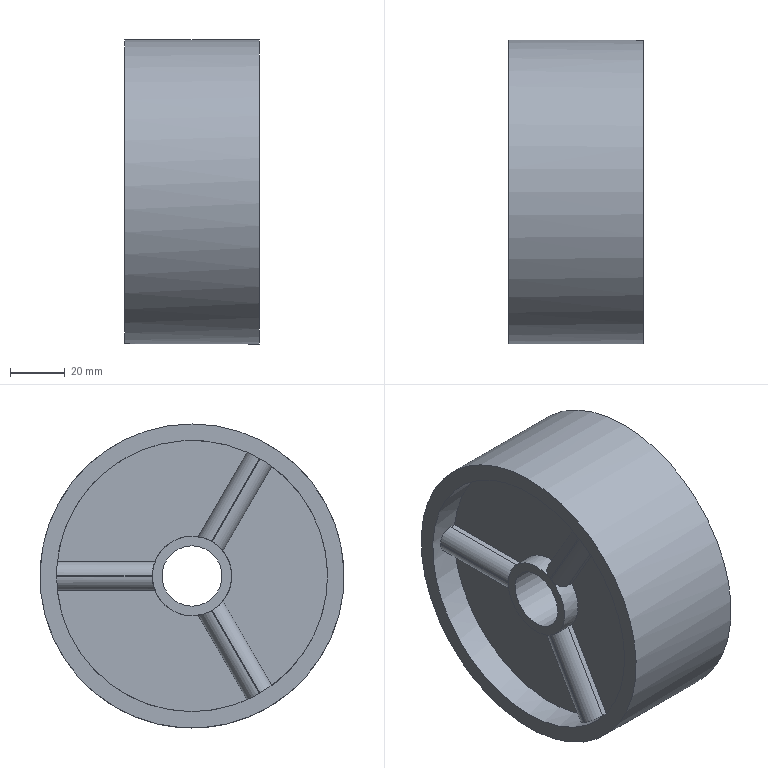Part | NX | features EXTRUDE 3, BLEND 1, DATUM_CSYS 1, EXTRACT_DATUM_PLANE 1, SKETCH 1, UNITE 1 | 1 solid | 44 faces | box 49 x 111 x 111 mm | volume 318902 mm3 | plane 22 | cylinder 22 | commonest cylinder face diameters 10 x12 29.03 x6 99 x2 22 x1 111 x1
STEP:
#1=CARTESIAN_POINT('',(-13.797,-29.113,40.033));
#2=VERTEX_POINT('',#1);
#3=CARTESIAN_POINT('',(-15.797,-29.113,40.033));
#4=VERTEX_POINT('',#3);
#5=CARTESIAN_POINT('',(21.203,-29.113,40.033));
#6=DIRECTION('',(-1.,0.,0.));
#7=VECTOR('',#6,1000.);
#8=LINE('',#5,#7);
#9=EDGE_CURVE('',#2,#4,#8,.T.);
#10=ORIENTED_EDGE('',*,*,#9,.T.);
#11=CARTESIAN_POINT('',(-15.797,-11.277,9.139));
#12=VERTEX_POINT('',#11);
#13=CARTESIAN_POINT('',(-15.797,-11.277,9.139));
#14=DIRECTION('',(0.,-0.5,0.866));
#15=VECTOR('',#14,1000.);
#16=LINE('',#13,#15);
#17=EDGE_CURVE('',#4,#12,#16,.F.);
#18=ORIENTED_EDGE('',*,*,#17,.T.);
#19=CARTESIAN_POINT('',(-13.797,-11.277,9.139));
#20=VERTEX_POINT('',#19);
#21=CARTESIAN_POINT('',(21.203,-11.277,9.139));
#22=DIRECTION('',(-1.,0.,0.));
#23=VECTOR('',#22,1000.);
#24=LINE('',#21,#23);
#25=EDGE_CURVE('',#20,#12,#24,.T.);
#26=ORIENTED_EDGE('',*,*,#25,.F.);
#27=CARTESIAN_POINT('',(-13.797,-29.113,40.033));
#28=DIRECTION('',(0.,0.5,-0.866));
#29=VECTOR('',#28,1000.);
#30=LINE('',#27,#29);
#31=EDGE_CURVE('',#2,#20,#30,.T.);
#32=ORIENTED_EDGE('',*,*,#31,.F.);
#33=EDGE_LOOP('',(#10,#18,#26,#32));
#34=FACE_BOUND('',#33,.T.);
#35=CARTESIAN_POINT('',(21.203,-11.277,9.139));
#36=DIRECTION('',(0.,-0.866,-0.5));
#37=DIRECTION('',(0.,0.5,-0.866));
#38=AXIS2_PLACEMENT_3D('',#35,#36,#37);
#39=PLANE('',#38);
#40=ADVANCED_FACE('',(#34),#39,.T.);
#41=CARTESIAN_POINT('',(-13.797,-11.277,-9.139));
#42=VERTEX_POINT('',#41);
#43=CARTESIAN_POINT('',(-15.797,-11.277,-9.139));
#44=VERTEX_POINT('',#43);
#45=CARTESIAN_POINT('',(21.203,-11.277,-9.139));
#46=DIRECTION('',(-1.,0.,0.));
#47=VECTOR('',#46,1000.);
#48=LINE('',#45,#47);
#49=EDGE_CURVE('',#42,#44,#48,.T.);
#50=ORIENTED_EDGE('',*,*,#49,.T.);
#51=CARTESIAN_POINT('',(-15.797,-29.113,-40.033));
#52=VERTEX_POINT('',#51);
#53=CARTESIAN_POINT('',(-15.797,-29.113,-40.033));
#54=DIRECTION('',(0.,0.5,0.866));
#55=VECTOR('',#54,1000.);
#56=LINE('',#53,#55);
#57=EDGE_CURVE('',#44,#52,#56,.F.);
#58=ORIENTED_EDGE('',*,*,#57,.T.);
#59=CARTESIAN_POINT('',(-13.797,-29.113,-40.033));
#60=VERTEX_POINT('',#59);
#61=CARTESIAN_POINT('',(21.203,-29.113,-40.033));
#62=DIRECTION('',(-1.,0.,0.));
#63=VECTOR('',#62,1000.);
#64=LINE('',#61,#63);
#65=EDGE_CURVE('',#60,#52,#64,.T.);
#66=ORIENTED_EDGE('',*,*,#65,.F.);
#67=CARTESIAN_POINT('',(-13.797,-11.277,-9.139));
#68=DIRECTION('',(0.,-0.5,-0.866));
#69=VECTOR('',#68,1000.);
#70=LINE('',#67,#69);
#71=EDGE_CURVE('',#42,#60,#70,.T.);
#72=ORIENTED_EDGE('',*,*,#71,.F.);
#73=EDGE_LOOP('',(#50,#58,#66,#72));
#74=FACE_BOUND('',#73,.T.);
#75=CARTESIAN_POINT('',(21.203,-29.113,-40.033));
#76=DIRECTION('',(0.,-0.866,0.5));
#77=DIRECTION('',(0.,-0.5,-0.866));
#78=AXIS2_PLACEMENT_3D('',#75,#76,#77);
#79=PLANE('',#78);
#80=ADVANCED_FACE('',(#74),#79,.T.);
#81=CARTESIAN_POINT('',(-24.797,0.,-49.5));
#82=VERTEX_POINT('',#81);
#83=CARTESIAN_POINT('',(-24.797,0.,0.));
#84=DIRECTION('',(1.,0.,0.));
#85=DIRECTION('',(0.,0.,-1.));
#86=AXIS2_PLACEMENT_3D('',#83,#84,#85);
#87=CIRCLE('',#86,49.5);
#88=EDGE_CURVE('',#82,#82,#87,.T.);
#89=ORIENTED_EDGE('',*,*,#88,.F.);
#90=EDGE_LOOP('',(#89));
#91=FACE_BOUND('',#90,.T.);
#92=CARTESIAN_POINT('',(-13.797,0.,0.));
#93=DIRECTION('',(-1.,0.,0.));
#94=DIRECTION('',(0.,0.,1.));
#95=AXIS2_PLACEMENT_3D('',#92,#93,#94);
#96=CIRCLE('',#95,49.5);
#97=EDGE_CURVE('',#60,#2,#96,.T.);
#98=ORIENTED_EDGE('',*,*,#97,.F.);
#99=ORIENTED_EDGE('',*,*,#65,.T.);
#100=CARTESIAN_POINT('',(-20.797,-24.92,-42.77));
#101=VERTEX_POINT('',#100);
#102=CARTESIAN_POINT('',(-15.797,-29.113,-40.033));
#103=CARTESIAN_POINT('',(-17.119,-29.113,-40.033));
#104=CARTESIAN_POINT('',(-19.705,-28.237,-40.691));
#105=CARTESIAN_POINT('',(-20.797,-26.062,-42.105));
#106=CARTESIAN_POINT('',(-20.797,-24.92,-42.77));
#107=B_SPLINE_CURVE_WITH_KNOTS('',3,(#102,#103,#104,#105,#106),.UNSPECIFIED.,.F.,.F.,(4,1,4),(0.,0.003908,0.007816),.UNSPECIFIED.);
#108=EDGE_CURVE('',#52,#101,#107,.T.);
#109=ORIENTED_EDGE('',*,*,#108,.T.);
#110=CARTESIAN_POINT('',(-20.797,-24.58,-42.966));
#111=VERTEX_POINT('',#110);
#112=CARTESIAN_POINT('',(-20.797,0.,0.));
#113=DIRECTION('',(-1.,0.,0.));
#114=DIRECTION('',(0.,0.,1.));
#115=AXIS2_PLACEMENT_3D('',#112,#113,#114);
#116=CIRCLE('',#115,49.5);
#117=EDGE_CURVE('',#111,#101,#116,.T.);
#118=ORIENTED_EDGE('',*,*,#117,.F.);
#119=CARTESIAN_POINT('',(-15.797,-20.113,-45.229));
#120=VERTEX_POINT('',#119);
#121=CARTESIAN_POINT('',(-20.797,-24.58,-42.966));
#122=CARTESIAN_POINT('',(-20.797,-23.433,-43.622));
#123=CARTESIAN_POINT('',(-19.71,-21.125,-44.797));
#124=CARTESIAN_POINT('',(-17.119,-20.113,-45.229));
#125=CARTESIAN_POINT('',(-15.797,-20.113,-45.229));
#126=B_SPLINE_CURVE_WITH_KNOTS('',3,(#121,#122,#123,#124,#125),.UNSPECIFIED.,.F.,.F.,(4,1,4),(0.,0.003908,0.007816),.UNSPECIFIED.);
#127=EDGE_CURVE('',#111,#120,#126,.T.);
#128=ORIENTED_EDGE('',*,*,#127,.T.);
#129=CARTESIAN_POINT('',(-13.797,-20.113,-45.229));
#130=VERTEX_POINT('',#129);
#131=CARTESIAN_POINT('',(21.203,-20.113,-45.229));
#132=DIRECTION('',(-1.,0.,0.));
#133=VECTOR('',#132,1000.);
#134=LINE('',#131,#133);
#135=EDGE_CURVE('',#130,#120,#134,.T.);
#136=ORIENTED_EDGE('',*,*,#135,.F.);
#137=CARTESIAN_POINT('',(-13.797,49.227,-5.196));
#138=VERTEX_POINT('',#137);
#139=CARTESIAN_POINT('',(-13.797,0.,0.));
#140=DIRECTION('',(-1.,0.,0.));
#141=DIRECTION('',(0.,0.,1.));
#142=AXIS2_PLACEMENT_3D('',#139,#140,#141);
#143=CIRCLE('',#142,49.5);
#144=EDGE_CURVE('',#138,#130,#143,.T.);
#145=ORIENTED_EDGE('',*,*,#144,.F.);
#146=CARTESIAN_POINT('',(-15.797,49.227,-5.196));
#147=VERTEX_POINT('',#146);
#148=CARTESIAN_POINT('',(21.203,49.227,-5.196));
#149=DIRECTION('',(-1.,0.,0.));
#150=VECTOR('',#149,1000.);
#151=LINE('',#148,#150);
#152=EDGE_CURVE('',#138,#147,#151,.T.);
#153=ORIENTED_EDGE('',*,*,#152,.T.);
#154=CARTESIAN_POINT('',(-20.797,49.5,-0.1962));
#155=VERTEX_POINT('',#154);
#156=CARTESIAN_POINT('',(-15.797,49.227,-5.196));
#157=CARTESIAN_POINT('',(-17.119,49.227,-5.196));
#158=CARTESIAN_POINT('',(-19.705,49.358,-4.109));
#159=CARTESIAN_POINT('',(-20.797,49.494,-1.518));
#160=CARTESIAN_POINT('',(-20.797,49.5,-0.1962));
#161=B_SPLINE_CURVE_WITH_KNOTS('',3,(#156,#157,#158,#159,#160),.UNSPECIFIED.,.F.,.F.,(4,1,4),(0.,0.003908,0.007816),.UNSPECIFIED.);
#162=EDGE_CURVE('',#147,#155,#161,.T.);
#163=ORIENTED_EDGE('',*,*,#162,.T.);
#164=CARTESIAN_POINT('',(-20.797,49.5,0.1962));
#165=VERTEX_POINT('',#164);
#166=CARTESIAN_POINT('',(-20.797,0.,0.));
#167=DIRECTION('',(-1.,0.,0.));
#168=DIRECTION('',(0.,0.,-1.));
#169=AXIS2_PLACEMENT_3D('',#166,#167,#168);
#170=CIRCLE('',#169,49.5);
#171=EDGE_CURVE('',#165,#155,#170,.T.);
#172=ORIENTED_EDGE('',*,*,#171,.F.);
#173=CARTESIAN_POINT('',(-15.797,49.227,5.196));
#174=VERTEX_POINT('',#173);
#175=CARTESIAN_POINT('',(-20.797,49.5,0.1962));
#176=CARTESIAN_POINT('',(-20.797,49.494,1.518));
#177=CARTESIAN_POINT('',(-19.71,49.358,4.104));
#178=CARTESIAN_POINT('',(-17.119,49.227,5.196));
#179=CARTESIAN_POINT('',(-15.797,49.227,5.196));
#180=B_SPLINE_CURVE_WITH_KNOTS('',3,(#175,#176,#177,#178,#179),.UNSPECIFIED.,.F.,.F.,(4,1,4),(0.,0.003908,0.007816),.UNSPECIFIED.);
#181=EDGE_CURVE('',#165,#174,#180,.T.);
#182=ORIENTED_EDGE('',*,*,#181,.T.);
#183=CARTESIAN_POINT('',(-13.797,49.227,5.196));
#184=VERTEX_POINT('',#183);
#185=CARTESIAN_POINT('',(21.203,49.227,5.196));
#186=DIRECTION('',(-1.,0.,0.));
#187=VECTOR('',#186,1000.);
#188=LINE('',#185,#187);
#189=EDGE_CURVE('',#184,#174,#188,.T.);
#190=ORIENTED_EDGE('',*,*,#189,.F.);
#191=CARTESIAN_POINT('',(-13.797,-20.113,45.229));
#192=VERTEX_POINT('',#191);
#193=CARTESIAN_POINT('',(-13.797,0.,0.));
#194=DIRECTION('',(-1.,0.,0.));
#195=DIRECTION('',(0.,0.,-1.));
#196=AXIS2_PLACEMENT_3D('',#193,#194,#195);
#197=CIRCLE('',#196,49.5);
#198=EDGE_CURVE('',#192,#184,#197,.T.);
#199=ORIENTED_EDGE('',*,*,#198,.F.);
#200=CARTESIAN_POINT('',(-15.797,-20.113,45.229));
#201=VERTEX_POINT('',#200);
#202=CARTESIAN_POINT('',(21.203,-20.113,45.229));
#203=DIRECTION('',(-1.,0.,0.));
#204=VECTOR('',#203,1000.);
#205=LINE('',#202,#204);
#206=EDGE_CURVE('',#192,#201,#205,.T.);
#207=ORIENTED_EDGE('',*,*,#206,.T.);
#208=CARTESIAN_POINT('',(-20.797,-24.58,42.966));
#209=VERTEX_POINT('',#208);
#210=CARTESIAN_POINT('',(-15.797,-20.113,45.229));
#211=CARTESIAN_POINT('',(-17.119,-20.113,45.229));
#212=CARTESIAN_POINT('',(-19.705,-21.121,44.799));
#213=CARTESIAN_POINT('',(-20.797,-23.433,43.622));
#214=CARTESIAN_POINT('',(-20.797,-24.58,42.966));
#215=B_SPLINE_CURVE_WITH_KNOTS('',3,(#210,#211,#212,#213,#214),.UNSPECIFIED.,.F.,.F.,(4,1,4),(0.,0.003908,0.007816),.UNSPECIFIED.);
#216=EDGE_CURVE('',#201,#209,#215,.T.);
#217=ORIENTED_EDGE('',*,*,#216,.T.);
#218=CARTESIAN_POINT('',(-20.797,-24.92,42.77));
#219=VERTEX_POINT('',#218);
#220=CARTESIAN_POINT('',(-20.797,0.,0.));
#221=DIRECTION('',(-1.,0.,0.));
#222=DIRECTION('',(0.,0.,1.));
#223=AXIS2_PLACEMENT_3D('',#220,#221,#222);
#224=CIRCLE('',#223,49.5);
#225=EDGE_CURVE('',#219,#209,#224,.T.);
#226=ORIENTED_EDGE('',*,*,#225,.F.);
#227=CARTESIAN_POINT('',(-20.797,-24.92,42.77));
#228=CARTESIAN_POINT('',(-20.797,-26.062,42.105));
#229=CARTESIAN_POINT('',(-19.71,-28.233,40.693));
#230=CARTESIAN_POINT('',(-17.119,-29.113,40.033));
#231=CARTESIAN_POINT('',(-15.797,-29.113,40.033));
#232=B_SPLINE_CURVE_WITH_KNOTS('',3,(#227,#228,#229,#230,#231),.UNSPECIFIED.,.F.,.F.,(4,1,4),(0.,0.003908,0.007816),.UNSPECIFIED.);
#233=EDGE_CURVE('',#219,#4,#232,.T.);
#234=ORIENTED_EDGE('',*,*,#233,.T.);
#235=ORIENTED_EDGE('',*,*,#9,.F.);
#236=EDGE_LOOP('',(#98,#99,#109,#118,#128,#136,#145,#153,#163,#172,#182,#190,#199,#207,#217,#226,#234,#235));
#237=FACE_BOUND('',#236,.T.);
#238=CARTESIAN_POINT('',(24.203,0.,0.));
#239=DIRECTION('',(-1.,0.,0.));
#240=DIRECTION('',(0.,0.,1.));
#241=AXIS2_PLACEMENT_3D('',#238,#239,#240);
#242=CYLINDRICAL_SURFACE('',#241,49.5);
#243=ADVANCED_FACE('',(#91,#237),#242,.F.);
#244=CARTESIAN_POINT('',(-13.797,0.,0.));
#245=DIRECTION('',(1.,0.,0.));
#246=DIRECTION('',(0.,-0.7769,0.6296));
#247=AXIS2_PLACEMENT_3D('',#244,#245,#246);
#248=CIRCLE('',#247,14.515);
#249=EDGE_CURVE('',#20,#42,#248,.T.);
#250=ORIENTED_EDGE('',*,*,#249,.F.);
#251=ORIENTED_EDGE('',*,*,#25,.T.);
#252=CARTESIAN_POINT('',(-20.797,-7.427,12.471));
#253=VERTEX_POINT('',#252);
#254=CARTESIAN_POINT('',(-15.797,-11.277,9.139));
#255=CARTESIAN_POINT('',(-17.131,-11.277,9.139));
#256=CARTESIAN_POINT('',(-19.701,-10.567,10.1));
#257=CARTESIAN_POINT('',(-20.797,-8.572,11.789));
#258=CARTESIAN_POINT('',(-20.797,-7.427,12.471));
#259=B_SPLINE_CURVE_WITH_KNOTS('',3,(#254,#255,#256,#257,#258),.UNSPECIFIED.,.F.,.F.,(4,1,4),(0.,0.00394,0.00788),.UNSPECIFIED.);
#260=EDGE_CURVE('',#12,#253,#259,.T.);
#261=ORIENTED_EDGE('',*,*,#260,.T.);
#262=CARTESIAN_POINT('',(-20.797,-7.427,-12.471));
#263=VERTEX_POINT('',#262);
#264=CARTESIAN_POINT('',(-20.797,0.,0.));
#265=DIRECTION('',(-1.,0.,0.));
#266=DIRECTION('',(0.,-0.7769,0.6296));
#267=AXIS2_PLACEMENT_3D('',#264,#265,#266);
#268=CIRCLE('',#267,14.515);
#269=EDGE_CURVE('',#263,#253,#268,.T.);
#270=ORIENTED_EDGE('',*,*,#269,.F.);
#271=CARTESIAN_POINT('',(-20.797,-7.427,-12.471));
#272=CARTESIAN_POINT('',(-20.797,-8.572,-11.789));
#273=CARTESIAN_POINT('',(-19.703,-10.565,-10.101));
#274=CARTESIAN_POINT('',(-17.131,-11.277,-9.139));
#275=CARTESIAN_POINT('',(-15.797,-11.277,-9.139));
#276=B_SPLINE_CURVE_WITH_KNOTS('',3,(#271,#272,#273,#274,#275),.UNSPECIFIED.,.F.,.F.,(4,1,4),(0.,0.00394,0.007881),.UNSPECIFIED.);
#277=EDGE_CURVE('',#263,#44,#276,.T.);
#278=ORIENTED_EDGE('',*,*,#277,.T.);
#279=ORIENTED_EDGE('',*,*,#49,.F.);
#280=EDGE_LOOP('',(#250,#251,#261,#270,#278,#279));
#281=FACE_BOUND('',#280,.T.);
#282=CARTESIAN_POINT('',(21.203,0.,0.));
#283=DIRECTION('',(-1.,0.,0.));
#284=DIRECTION('',(0.,0.,1.));
#285=AXIS2_PLACEMENT_3D('',#282,#283,#284);
#286=CYLINDRICAL_SURFACE('',#285,14.515);
#287=ADVANCED_FACE('',(#281),#286,.T.);
#288=CARTESIAN_POINT('',(-24.797,0.,55.5));
#289=VERTEX_POINT('',#288);
#290=CARTESIAN_POINT('',(-24.797,0.,0.));
#291=DIRECTION('',(-1.,0.,0.));
#292=DIRECTION('',(0.,0.,1.));
#293=AXIS2_PLACEMENT_3D('',#290,#291,#292);
#294=CIRCLE('',#293,55.5);
#295=EDGE_CURVE('',#289,#289,#294,.T.);
#296=ORIENTED_EDGE('',*,*,#295,.F.);
#297=EDGE_LOOP('',(#296));
#298=FACE_BOUND('',#297,.T.);
#299=CARTESIAN_POINT('',(24.203,0.,-55.5));
#300=VERTEX_POINT('',#299);
#301=CARTESIAN_POINT('',(24.203,0.,0.));
#302=DIRECTION('',(-1.,0.,0.));
#303=DIRECTION('',(0.,0.,-1.));
#304=AXIS2_PLACEMENT_3D('',#301,#302,#303);
#305=CIRCLE('',#304,55.5);
#306=EDGE_CURVE('',#300,#300,#305,.T.);
#307=ORIENTED_EDGE('',*,*,#306,.T.);
#308=EDGE_LOOP('',(#307));
#309=FACE_BOUND('',#308,.T.);
#310=CARTESIAN_POINT('',(24.203,0.,0.));
#311=DIRECTION('',(-1.,0.,0.));
#312=DIRECTION('',(0.,0.,1.));
#313=AXIS2_PLACEMENT_3D('',#310,#311,#312);
#314=CYLINDRICAL_SURFACE('',#313,55.5);
#315=ADVANCED_FACE('',(#298,#309),#314,.T.);
#316=CARTESIAN_POINT('',(21.203,-24.58,-42.966));
#317=VERTEX_POINT('',#316);
#318=CARTESIAN_POINT('',(21.203,-24.92,-42.77));
#319=VERTEX_POINT('',#318);
#320=CARTESIAN_POINT('',(21.203,0.,0.));
#321=DIRECTION('',(-1.,0.,0.));
#322=DIRECTION('',(0.,0.,1.));
#323=AXIS2_PLACEMENT_3D('',#320,#321,#322);
#324=CIRCLE('',#323,49.5);
#325=EDGE_CURVE('',#317,#319,#324,.T.);
#326=ORIENTED_EDGE('',*,*,#325,.T.);
#327=CARTESIAN_POINT('',(16.203,-29.113,-40.033));
#328=VERTEX_POINT('',#327);
#329=CARTESIAN_POINT('',(21.203,-24.92,-42.77));
#330=CARTESIAN_POINT('',(21.203,-26.062,-42.105));
#331=CARTESIAN_POINT('',(20.116,-28.233,-40.693));
#332=CARTESIAN_POINT('',(17.524,-29.113,-40.033));
#333=CARTESIAN_POINT('',(16.203,-29.113,-40.033));
#334=B_SPLINE_CURVE_WITH_KNOTS('',3,(#329,#330,#331,#332,#333),.UNSPECIFIED.,.F.,.F.,(4,1,4),(0.,0.003908,0.007816),.UNSPECIFIED.);
#335=EDGE_CURVE('',#319,#328,#334,.T.);
#336=ORIENTED_EDGE('',*,*,#335,.T.);
#337=CARTESIAN_POINT('',(14.203,-29.113,-40.033));
#338=VERTEX_POINT('',#337);
#339=CARTESIAN_POINT('',(21.203,-29.113,-40.033));
#340=DIRECTION('',(-1.,0.,0.));
#341=VECTOR('',#340,1000.);
#342=LINE('',#339,#341);
#343=EDGE_CURVE('',#328,#338,#342,.T.);
#344=ORIENTED_EDGE('',*,*,#343,.T.);
#345=CARTESIAN_POINT('',(14.203,-29.113,40.033));
#346=VERTEX_POINT('',#345);
#347=CARTESIAN_POINT('',(14.203,0.,0.));
#348=DIRECTION('',(-1.,0.,0.));
#349=DIRECTION('',(0.,0.,1.));
#350=AXIS2_PLACEMENT_3D('',#347,#348,#349);
#351=CIRCLE('',#350,49.5);
#352=EDGE_CURVE('',#338,#346,#351,.T.);
#353=ORIENTED_EDGE('',*,*,#352,.T.);
#354=CARTESIAN_POINT('',(16.203,-29.113,40.033));
#355=VERTEX_POINT('',#354);
#356=CARTESIAN_POINT('',(21.203,-29.113,40.033));
#357=DIRECTION('',(-1.,0.,0.));
#358=VECTOR('',#357,1000.);
#359=LINE('',#356,#358);
#360=EDGE_CURVE('',#355,#346,#359,.T.);
#361=ORIENTED_EDGE('',*,*,#360,.F.);
#362=CARTESIAN_POINT('',(21.203,-24.92,42.77));
#363=VERTEX_POINT('',#362);
#364=CARTESIAN_POINT('',(16.203,-29.113,40.033));
#365=CARTESIAN_POINT('',(17.524,-29.113,40.033));
#366=CARTESIAN_POINT('',(20.111,-28.237,40.691));
#367=CARTESIAN_POINT('',(21.203,-26.062,42.105));
#368=CARTESIAN_POINT('',(21.203,-24.92,42.77));
#369=B_SPLINE_CURVE_WITH_KNOTS('',3,(#364,#365,#366,#367,#368),.UNSPECIFIED.,.F.,.F.,(4,1,4),(0.,0.003908,0.007816),.UNSPECIFIED.);
#370=EDGE_CURVE('',#355,#363,#369,.T.);
#371=ORIENTED_EDGE('',*,*,#370,.T.);
#372=CARTESIAN_POINT('',(21.203,-24.58,42.966));
#373=VERTEX_POINT('',#372);
#374=CARTESIAN_POINT('',(21.203,0.,0.));
#375=DIRECTION('',(-1.,0.,0.));
#376=DIRECTION('',(0.,0.,1.));
#377=AXIS2_PLACEMENT_3D('',#374,#375,#376);
#378=CIRCLE('',#377,49.5);
#379=EDGE_CURVE('',#363,#373,#378,.T.);
#380=ORIENTED_EDGE('',*,*,#379,.T.);
#381=CARTESIAN_POINT('',(16.203,-20.113,45.229));
#382=VERTEX_POINT('',#381);
#383=CARTESIAN_POINT('',(21.203,-24.58,42.966));
#384=CARTESIAN_POINT('',(21.203,-23.433,43.622));
#385=CARTESIAN_POINT('',(20.116,-21.125,44.797));
#386=CARTESIAN_POINT('',(17.524,-20.113,45.229));
#387=CARTESIAN_POINT('',(16.203,-20.113,45.229));
#388=B_SPLINE_CURVE_WITH_KNOTS('',3,(#383,#384,#385,#386,#387),.UNSPECIFIED.,.F.,.F.,(4,1,4),(0.,0.003908,0.007816),.UNSPECIFIED.);
#389=EDGE_CURVE('',#373,#382,#388,.T.);
#390=ORIENTED_EDGE('',*,*,#389,.T.);
#391=CARTESIAN_POINT('',(14.203,-20.113,45.229));
#392=VERTEX_POINT('',#391);
#393=CARTESIAN_POINT('',(21.203,-20.113,45.229));
#394=DIRECTION('',(-1.,0.,0.));
#395=VECTOR('',#394,1000.);
#396=LINE('',#393,#395);
#397=EDGE_CURVE('',#382,#392,#396,.T.);
#398=ORIENTED_EDGE('',*,*,#397,.T.);
#399=CARTESIAN_POINT('',(14.203,49.227,5.196));
#400=VERTEX_POINT('',#399);
#401=CARTESIAN_POINT('',(14.203,0.,0.));
#402=DIRECTION('',(-1.,0.,0.));
#403=DIRECTION('',(0.,0.,1.));
#404=AXIS2_PLACEMENT_3D('',#401,#402,#403);
#405=CIRCLE('',#404,49.5);
#406=EDGE_CURVE('',#392,#400,#405,.T.);
#407=ORIENTED_EDGE('',*,*,#406,.T.);
#408=CARTESIAN_POINT('',(16.203,49.227,5.196));
#409=VERTEX_POINT('',#408);
#410=CARTESIAN_POINT('',(21.203,49.227,5.196));
#411=DIRECTION('',(-1.,0.,0.));
#412=VECTOR('',#411,1000.);
#413=LINE('',#410,#412);
#414=EDGE_CURVE('',#409,#400,#413,.T.);
#415=ORIENTED_EDGE('',*,*,#414,.F.);
#416=CARTESIAN_POINT('',(21.203,49.5,0.1962));
#417=VERTEX_POINT('',#416);
#418=CARTESIAN_POINT('',(16.203,49.227,5.196));
#419=CARTESIAN_POINT('',(17.524,49.227,5.196));
#420=CARTESIAN_POINT('',(20.111,49.358,4.109));
#421=CARTESIAN_POINT('',(21.203,49.494,1.518));
#422=CARTESIAN_POINT('',(21.203,49.5,0.1962));
#423=B_SPLINE_CURVE_WITH_KNOTS('',3,(#418,#419,#420,#421,#422),.UNSPECIFIED.,.F.,.F.,(4,1,4),(0.,0.003908,0.007816),.UNSPECIFIED.);
#424=EDGE_CURVE('',#409,#417,#423,.T.);
#425=ORIENTED_EDGE('',*,*,#424,.T.);
#426=CARTESIAN_POINT('',(21.203,49.5,-0.1962));
#427=VERTEX_POINT('',#426);
#428=CARTESIAN_POINT('',(21.203,0.,0.));
#429=DIRECTION('',(-1.,0.,0.));
#430=DIRECTION('',(0.,0.,-1.));
#431=AXIS2_PLACEMENT_3D('',#428,#429,#430);
#432=CIRCLE('',#431,49.5);
#433=EDGE_CURVE('',#417,#427,#432,.T.);
#434=ORIENTED_EDGE('',*,*,#433,.T.);
#435=CARTESIAN_POINT('',(16.203,49.227,-5.196));
#436=VERTEX_POINT('',#435);
#437=CARTESIAN_POINT('',(21.203,49.5,-0.1962));
#438=CARTESIAN_POINT('',(21.203,49.494,-1.518));
#439=CARTESIAN_POINT('',(20.116,49.358,-4.104));
#440=CARTESIAN_POINT('',(17.524,49.227,-5.196));
#441=CARTESIAN_POINT('',(16.203,49.227,-5.196));
#442=B_SPLINE_CURVE_WITH_KNOTS('',3,(#437,#438,#439,#440,#441),.UNSPECIFIED.,.F.,.F.,(4,1,4),(0.,0.003908,0.007816),.UNSPECIFIED.);
#443=EDGE_CURVE('',#427,#436,#442,.T.);
#444=ORIENTED_EDGE('',*,*,#443,.T.);
#445=CARTESIAN_POINT('',(14.203,49.227,-5.196));
#446=VERTEX_POINT('',#445);
#447=CARTESIAN_POINT('',(21.203,49.227,-5.196));
#448=DIRECTION('',(-1.,0.,0.));
#449=VECTOR('',#448,1000.);
#450=LINE('',#447,#449);
#451=EDGE_CURVE('',#436,#446,#450,.T.);
#452=ORIENTED_EDGE('',*,*,#451,.T.);
#453=CARTESIAN_POINT('',(14.203,-20.113,-45.229));
#454=VERTEX_POINT('',#453);
#455=CARTESIAN_POINT('',(14.203,0.,0.));
#456=DIRECTION('',(-1.,0.,0.));
#457=DIRECTION('',(0.,0.,-1.));
#458=AXIS2_PLACEMENT_3D('',#455,#456,#457);
#459=CIRCLE('',#458,49.5);
#460=EDGE_CURVE('',#446,#454,#459,.T.);
#461=ORIENTED_EDGE('',*,*,#460,.T.);
#462=CARTESIAN_POINT('',(16.203,-20.113,-45.229));
#463=VERTEX_POINT('',#462);
#464=CARTESIAN_POINT('',(21.203,-20.113,-45.229));
#465=DIRECTION('',(-1.,0.,0.));
#466=VECTOR('',#465,1000.);
#467=LINE('',#464,#466);
#468=EDGE_CURVE('',#463,#454,#467,.T.);
#469=ORIENTED_EDGE('',*,*,#468,.F.);
#470=CARTESIAN_POINT('',(16.203,-20.113,-45.229));
#471=CARTESIAN_POINT('',(17.524,-20.113,-45.229));
#472=CARTESIAN_POINT('',(20.111,-21.121,-44.799));
#473=CARTESIAN_POINT('',(21.203,-23.433,-43.622));
#474=CARTESIAN_POINT('',(21.203,-24.58,-42.966));
#475=B_SPLINE_CURVE_WITH_KNOTS('',3,(#470,#471,#472,#473,#474),.UNSPECIFIED.,.F.,.F.,(4,1,4),(0.,0.003908,0.007816),.UNSPECIFIED.);
#476=EDGE_CURVE('',#463,#317,#475,.T.);
#477=ORIENTED_EDGE('',*,*,#476,.T.);
#478=EDGE_LOOP('',(#326,#336,#344,#353,#361,#371,#380,#390,#398,#407,#415,#425,#434,#444,#452,#461,#469,#477));
#479=FACE_BOUND('',#478,.T.);
#480=CARTESIAN_POINT('',(24.203,0.,49.5));
#481=VERTEX_POINT('',#480);
#482=CARTESIAN_POINT('',(24.203,0.,0.));
#483=DIRECTION('',(1.,0.,0.));
#484=DIRECTION('',(0.,0.,1.));
#485=AXIS2_PLACEMENT_3D('',#482,#483,#484);
#486=CIRCLE('',#485,49.5);
#487=EDGE_CURVE('',#481,#481,#486,.T.);
#488=ORIENTED_EDGE('',*,*,#487,.T.);
#489=EDGE_LOOP('',(#488));
#490=FACE_BOUND('',#489,.T.);
#491=CARTESIAN_POINT('',(24.203,0.,0.));
#492=DIRECTION('',(-1.,0.,0.));
#493=DIRECTION('',(0.,0.,1.));
#494=AXIS2_PLACEMENT_3D('',#491,#492,#493);
#495=CYLINDRICAL_SURFACE('',#494,49.5);
#496=ADVANCED_FACE('',(#479,#490),#495,.F.);
#497=ORIENTED_EDGE('',*,*,#306,.F.);
#498=EDGE_LOOP('',(#497));
#499=FACE_BOUND('',#498,.T.);
#500=ORIENTED_EDGE('',*,*,#487,.F.);
#501=EDGE_LOOP('',(#500));
#502=FACE_BOUND('',#501,.T.);
#503=CARTESIAN_POINT('',(24.203,0.,0.));
#504=DIRECTION('',(-1.,0.,0.));
#505=DIRECTION('',(0.,0.,1.));
#506=AXIS2_PLACEMENT_3D('',#503,#504,#505);
#507=PLANE('',#506);
#508=ADVANCED_FACE('',(#499,#502),#507,.F.);
#509=ORIENTED_EDGE('',*,*,#295,.T.);
#510=EDGE_LOOP('',(#509));
#511=FACE_BOUND('',#510,.T.);
#512=ORIENTED_EDGE('',*,*,#88,.T.);
#513=EDGE_LOOP('',(#512));
#514=FACE_BOUND('',#513,.T.);
#515=CARTESIAN_POINT('',(-24.797,0.,0.));
#516=DIRECTION('',(-1.,0.,0.));
#517=DIRECTION('',(0.,0.,1.));
#518=AXIS2_PLACEMENT_3D('',#515,#516,#517);
#519=PLANE('',#518);
#520=ADVANCED_FACE('',(#511,#514),#519,.T.);
#521=ORIENTED_EDGE('',*,*,#397,.F.);
#522=CARTESIAN_POINT('',(16.203,-2.277,14.336));
#523=VERTEX_POINT('',#522);
#524=CARTESIAN_POINT('',(16.203,-2.277,14.336));
#525=DIRECTION('',(0.,0.5,-0.866));
#526=VECTOR('',#525,1000.);
#527=LINE('',#524,#526);
#528=EDGE_CURVE('',#382,#523,#527,.T.);
#529=ORIENTED_EDGE('',*,*,#528,.T.);
#530=CARTESIAN_POINT('',(14.203,-2.277,14.336));
#531=VERTEX_POINT('',#530);
#532=CARTESIAN_POINT('',(21.203,-2.277,14.336));
#533=DIRECTION('',(-1.,0.,0.));
#534=VECTOR('',#533,1000.);
#535=LINE('',#532,#534);
#536=EDGE_CURVE('',#523,#531,#535,.T.);
#537=ORIENTED_EDGE('',*,*,#536,.T.);
#538=CARTESIAN_POINT('',(14.203,-2.277,14.336));
#539=DIRECTION('',(0.,-0.5,0.866));
#540=VECTOR('',#539,1000.);
#541=LINE('',#538,#540);
#542=EDGE_CURVE('',#531,#392,#541,.T.);
#543=ORIENTED_EDGE('',*,*,#542,.T.);
#544=EDGE_LOOP('',(#521,#529,#537,#543));
#545=FACE_BOUND('',#544,.T.);
#546=CARTESIAN_POINT('',(21.203,-20.113,45.229));
#547=DIRECTION('',(0.,0.866,0.5));
#548=DIRECTION('',(0.,-0.5,0.866));
#549=AXIS2_PLACEMENT_3D('',#546,#547,#548);
#550=PLANE('',#549);
#551=ADVANCED_FACE('',(#545),#550,.T.);
#552=CARTESIAN_POINT('',(16.203,13.553,5.196));
#553=VERTEX_POINT('',#552);
#554=CARTESIAN_POINT('',(14.203,13.553,5.196));
#555=VERTEX_POINT('',#554);
#556=CARTESIAN_POINT('',(21.203,13.553,5.196));
#557=DIRECTION('',(-1.,0.,0.));
#558=VECTOR('',#557,1000.);
#559=LINE('',#556,#558);
#560=EDGE_CURVE('',#553,#555,#559,.T.);
#561=ORIENTED_EDGE('',*,*,#560,.F.);
#562=CARTESIAN_POINT('',(16.203,49.227,5.196));
#563=DIRECTION('',(0.,1.,0.));
#564=VECTOR('',#563,1000.);
#565=LINE('',#562,#564);
#566=EDGE_CURVE('',#553,#409,#565,.T.);
#567=ORIENTED_EDGE('',*,*,#566,.T.);
#568=ORIENTED_EDGE('',*,*,#414,.T.);
#569=CARTESIAN_POINT('',(14.203,49.227,5.196));
#570=DIRECTION('',(0.,-1.,0.));
#571=VECTOR('',#570,1000.);
#572=LINE('',#569,#571);
#573=EDGE_CURVE('',#400,#555,#572,.T.);
#574=ORIENTED_EDGE('',*,*,#573,.T.);
#575=EDGE_LOOP('',(#561,#567,#568,#574));
#576=FACE_BOUND('',#575,.T.);
#577=CARTESIAN_POINT('',(21.203,13.553,5.196));
#578=DIRECTION('',(0.,0.,1.));
#579=DIRECTION('',(1.,0.,0.));
#580=AXIS2_PLACEMENT_3D('',#577,#578,#579);
#581=PLANE('',#580);
#582=ADVANCED_FACE('',(#576),#581,.T.);
#583=CARTESIAN_POINT('',(21.203,-7.087,12.667));
#584=VERTEX_POINT('',#583);
#585=CARTESIAN_POINT('',(21.203,14.514,0.1962));
#586=VERTEX_POINT('',#585);
#587=CARTESIAN_POINT('',(21.203,0.,0.));
#588=DIRECTION('',(-1.,0.,0.));
#589=DIRECTION('',(0.,0.,1.));
#590=AXIS2_PLACEMENT_3D('',#587,#588,#589);
#591=CIRCLE('',#590,14.515);
#592=EDGE_CURVE('',#584,#586,#591,.T.);
#593=ORIENTED_EDGE('',*,*,#592,.T.);
#594=CARTESIAN_POINT('',(21.203,14.514,0.1962));
#595=CARTESIAN_POINT('',(21.203,14.496,1.529));
#596=CARTESIAN_POINT('',(20.109,14.031,4.099));
#597=CARTESIAN_POINT('',(17.536,13.553,5.196));
#598=CARTESIAN_POINT('',(16.203,13.553,5.196));
#599=B_SPLINE_CURVE_WITH_KNOTS('',3,(#594,#595,#596,#597,#598),.UNSPECIFIED.,.F.,.F.,(4,1,4),(0.,0.00394,0.007881),.UNSPECIFIED.);
#600=EDGE_CURVE('',#586,#553,#599,.T.);
#601=ORIENTED_EDGE('',*,*,#600,.T.);
#602=ORIENTED_EDGE('',*,*,#560,.T.);
#603=CARTESIAN_POINT('',(14.203,0.,0.));
#604=DIRECTION('',(1.,0.,0.));
#605=DIRECTION('',(0.,0.9337,0.358));
#606=AXIS2_PLACEMENT_3D('',#603,#604,#605);
#607=CIRCLE('',#606,14.515);
#608=EDGE_CURVE('',#555,#531,#607,.T.);
#609=ORIENTED_EDGE('',*,*,#608,.T.);
#610=ORIENTED_EDGE('',*,*,#536,.F.);
#611=CARTESIAN_POINT('',(16.203,-2.277,14.336));
#612=CARTESIAN_POINT('',(17.536,-2.277,14.336));
#613=CARTESIAN_POINT('',(20.106,-3.463,14.201));
#614=CARTESIAN_POINT('',(21.203,-5.924,13.318));
#615=CARTESIAN_POINT('',(21.203,-7.087,12.667));
#616=B_SPLINE_CURVE_WITH_KNOTS('',3,(#611,#612,#613,#614,#615),.UNSPECIFIED.,.F.,.F.,(4,1,4),(0.,0.00394,0.00788),.UNSPECIFIED.);
#617=EDGE_CURVE('',#523,#584,#616,.T.);
#618=ORIENTED_EDGE('',*,*,#617,.T.);
#619=EDGE_LOOP('',(#593,#601,#602,#609,#610,#618));
#620=FACE_BOUND('',#619,.T.);
#621=CARTESIAN_POINT('',(21.203,0.,0.));
#622=DIRECTION('',(-1.,0.,0.));
#623=DIRECTION('',(0.,0.,1.));
#624=AXIS2_PLACEMENT_3D('',#621,#622,#623);
#625=CYLINDRICAL_SURFACE('',#624,14.515);
#626=ADVANCED_FACE('',(#620),#625,.T.);
#627=ORIENTED_EDGE('',*,*,#451,.F.);
#628=CARTESIAN_POINT('',(16.203,13.553,-5.196));
#629=VERTEX_POINT('',#628);
#630=CARTESIAN_POINT('',(16.203,13.553,-5.196));
#631=DIRECTION('',(0.,-1.,0.));
#632=VECTOR('',#631,1000.);
#633=LINE('',#630,#632);
#634=EDGE_CURVE('',#436,#629,#633,.T.);
#635=ORIENTED_EDGE('',*,*,#634,.T.);
#636=CARTESIAN_POINT('',(14.203,13.553,-5.196));
#637=VERTEX_POINT('',#636);
#638=CARTESIAN_POINT('',(21.203,13.553,-5.196));
#639=DIRECTION('',(-1.,0.,0.));
#640=VECTOR('',#639,1000.);
#641=LINE('',#638,#640);
#642=EDGE_CURVE('',#629,#637,#641,.T.);
#643=ORIENTED_EDGE('',*,*,#642,.T.);
#644=CARTESIAN_POINT('',(14.203,13.553,-5.196));
#645=DIRECTION('',(0.,1.,0.));
#646=VECTOR('',#645,1000.);
#647=LINE('',#644,#646);
#648=EDGE_CURVE('',#637,#446,#647,.T.);
#649=ORIENTED_EDGE('',*,*,#648,.T.);
#650=EDGE_LOOP('',(#627,#635,#643,#649));
#651=FACE_BOUND('',#650,.T.);
#652=CARTESIAN_POINT('',(21.203,49.227,-5.196));
#653=DIRECTION('',(0.,0.,-1.));
#654=DIRECTION('',(-1.,0.,0.));
#655=AXIS2_PLACEMENT_3D('',#652,#653,#654);
#656=PLANE('',#655);
#657=ADVANCED_FACE('',(#651),#656,.T.);
#658=CARTESIAN_POINT('',(16.203,-2.277,-14.336));
#659=VERTEX_POINT('',#658);
#660=CARTESIAN_POINT('',(14.203,-2.277,-14.336));
#661=VERTEX_POINT('',#660);
#662=CARTESIAN_POINT('',(21.203,-2.277,-14.336));
#663=DIRECTION('',(-1.,0.,0.));
#664=VECTOR('',#663,1000.);
#665=LINE('',#662,#664);
#666=EDGE_CURVE('',#659,#661,#665,.T.);
#667=ORIENTED_EDGE('',*,*,#666,.F.);
#668=CARTESIAN_POINT('',(16.203,-20.113,-45.229));
#669=DIRECTION('',(0.,-0.5,-0.866));
#670=VECTOR('',#669,1000.);
#671=LINE('',#668,#670);
#672=EDGE_CURVE('',#659,#463,#671,.T.);
#673=ORIENTED_EDGE('',*,*,#672,.T.);
#674=ORIENTED_EDGE('',*,*,#468,.T.);
#675=CARTESIAN_POINT('',(14.203,-20.113,-45.229));
#676=DIRECTION('',(0.,0.5,0.866));
#677=VECTOR('',#676,1000.);
#678=LINE('',#675,#677);
#679=EDGE_CURVE('',#454,#661,#678,.T.);
#680=ORIENTED_EDGE('',*,*,#679,.T.);
#681=EDGE_LOOP('',(#667,#673,#674,#680));
#682=FACE_BOUND('',#681,.T.);
#683=CARTESIAN_POINT('',(21.203,-2.277,-14.336));
#684=DIRECTION('',(0.,0.866,-0.5));
#685=DIRECTION('',(0.,0.5,0.866));
#686=AXIS2_PLACEMENT_3D('',#683,#684,#685);
#687=PLANE('',#686);
#688=ADVANCED_FACE('',(#682),#687,.T.);
#689=CARTESIAN_POINT('',(21.203,14.514,-0.1962));
#690=VERTEX_POINT('',#689);
#691=CARTESIAN_POINT('',(21.203,-7.087,-12.667));
#692=VERTEX_POINT('',#691);
#693=CARTESIAN_POINT('',(21.203,0.,0.));
#694=DIRECTION('',(-1.,0.,0.));
#695=DIRECTION('',(0.,0.,-1.));
#696=AXIS2_PLACEMENT_3D('',#693,#694,#695);
#697=CIRCLE('',#696,14.515);
#698=EDGE_CURVE('',#690,#692,#697,.T.);
#699=ORIENTED_EDGE('',*,*,#698,.T.);
#700=CARTESIAN_POINT('',(21.203,-7.087,-12.667));
#701=CARTESIAN_POINT('',(21.203,-5.924,-13.318));
#702=CARTESIAN_POINT('',(20.109,-3.465,-14.2));
#703=CARTESIAN_POINT('',(17.536,-2.277,-14.336));
#704=CARTESIAN_POINT('',(16.203,-2.277,-14.336));
#705=B_SPLINE_CURVE_WITH_KNOTS('',3,(#700,#701,#702,#703,#704),.UNSPECIFIED.,.F.,.F.,(4,1,4),(0.,0.00394,0.007881),.UNSPECIFIED.);
#706=EDGE_CURVE('',#692,#659,#705,.T.);
#707=ORIENTED_EDGE('',*,*,#706,.T.);
#708=ORIENTED_EDGE('',*,*,#666,.T.);
#709=CARTESIAN_POINT('',(14.203,0.,0.));
#710=DIRECTION('',(1.,0.,0.));
#711=DIRECTION('',(0.,-0.1568,-0.9876));
#712=AXIS2_PLACEMENT_3D('',#709,#710,#711);
#713=CIRCLE('',#712,14.515);
#714=EDGE_CURVE('',#661,#637,#713,.T.);
#715=ORIENTED_EDGE('',*,*,#714,.T.);
#716=ORIENTED_EDGE('',*,*,#642,.F.);
#717=CARTESIAN_POINT('',(16.203,13.553,-5.196));
#718=CARTESIAN_POINT('',(17.536,13.553,-5.196));
#719=CARTESIAN_POINT('',(20.106,14.03,-4.101));
#720=CARTESIAN_POINT('',(21.203,14.496,-1.529));
#721=CARTESIAN_POINT('',(21.203,14.514,-0.1962));
#722=B_SPLINE_CURVE_WITH_KNOTS('',3,(#717,#718,#719,#720,#721),.UNSPECIFIED.,.F.,.F.,(4,1,4),(0.,0.00394,0.00788),.UNSPECIFIED.);
#723=EDGE_CURVE('',#629,#690,#722,.T.);
#724=ORIENTED_EDGE('',*,*,#723,.T.);
#725=EDGE_LOOP('',(#699,#707,#708,#715,#716,#724));
#726=FACE_BOUND('',#725,.T.);
#727=CARTESIAN_POINT('',(21.203,0.,0.));
#728=DIRECTION('',(-1.,0.,0.));
#729=DIRECTION('',(0.,0.,1.));
#730=AXIS2_PLACEMENT_3D('',#727,#728,#729);
#731=CYLINDRICAL_SURFACE('',#730,14.515);
#732=ADVANCED_FACE('',(#726),#731,.T.);
#733=ORIENTED_EDGE('',*,*,#343,.F.);
#734=CARTESIAN_POINT('',(16.203,-11.277,-9.139));
#735=VERTEX_POINT('',#734);
#736=CARTESIAN_POINT('',(16.203,-11.277,-9.139));
#737=DIRECTION('',(0.,0.5,0.866));
#738=VECTOR('',#737,1000.);
#739=LINE('',#736,#738);
#740=EDGE_CURVE('',#328,#735,#739,.T.);
#741=ORIENTED_EDGE('',*,*,#740,.T.);
#742=CARTESIAN_POINT('',(14.203,-11.277,-9.139));
#743=VERTEX_POINT('',#742);
#744=CARTESIAN_POINT('',(21.203,-11.277,-9.139));
#745=DIRECTION('',(-1.,0.,0.));
#746=VECTOR('',#745,1000.);
#747=LINE('',#744,#746);
#748=EDGE_CURVE('',#735,#743,#747,.T.);
#749=ORIENTED_EDGE('',*,*,#748,.T.);
#750=CARTESIAN_POINT('',(14.203,-11.277,-9.139));
#751=DIRECTION('',(0.,-0.5,-0.866));
#752=VECTOR('',#751,1000.);
#753=LINE('',#750,#752);
#754=EDGE_CURVE('',#743,#338,#753,.T.);
#755=ORIENTED_EDGE('',*,*,#754,.T.);
#756=EDGE_LOOP('',(#733,#741,#749,#755));
#757=FACE_BOUND('',#756,.T.);
#758=CARTESIAN_POINT('',(21.203,-29.113,-40.033));
#759=DIRECTION('',(0.,-0.866,0.5));
#760=DIRECTION('',(0.,-0.5,-0.866));
#761=AXIS2_PLACEMENT_3D('',#758,#759,#760);
#762=PLANE('',#761);
#763=ADVANCED_FACE('',(#757),#762,.T.);
#764=CARTESIAN_POINT('',(21.203,-7.427,-12.471));
#765=VERTEX_POINT('',#764);
#766=CARTESIAN_POINT('',(21.203,-7.427,12.471));
#767=VERTEX_POINT('',#766);
#768=CARTESIAN_POINT('',(21.203,0.,0.));
#769=DIRECTION('',(-1.,0.,0.));
#770=DIRECTION('',(0.,-0.7769,0.6296));
#771=AXIS2_PLACEMENT_3D('',#768,#769,#770);
#772=CIRCLE('',#771,14.515);
#773=EDGE_CURVE('',#765,#767,#772,.T.);
#774=ORIENTED_EDGE('',*,*,#773,.T.);
#775=CARTESIAN_POINT('',(16.203,-11.277,9.139));
#776=VERTEX_POINT('',#775);
#777=CARTESIAN_POINT('',(21.203,-7.427,12.471));
#778=CARTESIAN_POINT('',(21.203,-8.572,11.789));
#779=CARTESIAN_POINT('',(20.109,-10.565,10.101));
#780=CARTESIAN_POINT('',(17.536,-11.277,9.139));
#781=CARTESIAN_POINT('',(16.203,-11.277,9.139));
#782=B_SPLINE_CURVE_WITH_KNOTS('',3,(#777,#778,#779,#780,#781),.UNSPECIFIED.,.F.,.F.,(4,1,4),(0.,0.00394,0.007881),.UNSPECIFIED.);
#783=EDGE_CURVE('',#767,#776,#782,.T.);
#784=ORIENTED_EDGE('',*,*,#783,.T.);
#785=CARTESIAN_POINT('',(14.203,-11.277,9.139));
#786=VERTEX_POINT('',#785);
#787=CARTESIAN_POINT('',(21.203,-11.277,9.139));
#788=DIRECTION('',(-1.,0.,0.));
#789=VECTOR('',#788,1000.);
#790=LINE('',#787,#789);
#791=EDGE_CURVE('',#776,#786,#790,.T.);
#792=ORIENTED_EDGE('',*,*,#791,.T.);
#793=CARTESIAN_POINT('',(14.203,0.,0.));
#794=DIRECTION('',(1.,0.,0.));
#795=DIRECTION('',(0.,-0.7769,0.6296));
#796=AXIS2_PLACEMENT_3D('',#793,#794,#795);
#797=CIRCLE('',#796,14.515);
#798=EDGE_CURVE('',#786,#743,#797,.T.);
#799=ORIENTED_EDGE('',*,*,#798,.T.);
#800=ORIENTED_EDGE('',*,*,#748,.F.);
#801=CARTESIAN_POINT('',(16.203,-11.277,-9.139));
#802=CARTESIAN_POINT('',(17.536,-11.277,-9.139));
#803=CARTESIAN_POINT('',(20.106,-10.567,-10.1));
#804=CARTESIAN_POINT('',(21.203,-8.572,-11.789));
#805=CARTESIAN_POINT('',(21.203,-7.427,-12.471));
#806=B_SPLINE_CURVE_WITH_KNOTS('',3,(#801,#802,#803,#804,#805),.UNSPECIFIED.,.F.,.F.,(4,1,4),(0.,0.00394,0.00788),.UNSPECIFIED.);
#807=EDGE_CURVE('',#735,#765,#806,.T.);
#808=ORIENTED_EDGE('',*,*,#807,.T.);
#809=EDGE_LOOP('',(#774,#784,#792,#799,#800,#808));
#810=FACE_BOUND('',#809,.T.);
#811=CARTESIAN_POINT('',(21.203,0.,0.));
#812=DIRECTION('',(-1.,0.,0.));
#813=DIRECTION('',(0.,0.,1.));
#814=AXIS2_PLACEMENT_3D('',#811,#812,#813);
#815=CYLINDRICAL_SURFACE('',#814,14.515);
#816=ADVANCED_FACE('',(#810),#815,.T.);
#817=ORIENTED_EDGE('',*,*,#791,.F.);
#818=CARTESIAN_POINT('',(16.203,-29.113,40.033));
#819=DIRECTION('',(0.,-0.5,0.866));
#820=VECTOR('',#819,1000.);
#821=LINE('',#818,#820);
#822=EDGE_CURVE('',#776,#355,#821,.T.);
#823=ORIENTED_EDGE('',*,*,#822,.T.);
#824=ORIENTED_EDGE('',*,*,#360,.T.);
#825=CARTESIAN_POINT('',(14.203,-29.113,40.033));
#826=DIRECTION('',(0.,0.5,-0.866));
#827=VECTOR('',#826,1000.);
#828=LINE('',#825,#827);
#829=EDGE_CURVE('',#346,#786,#828,.T.);
#830=ORIENTED_EDGE('',*,*,#829,.T.);
#831=EDGE_LOOP('',(#817,#823,#824,#830));
#832=FACE_BOUND('',#831,.T.);
#833=CARTESIAN_POINT('',(21.203,-11.277,9.139));
#834=DIRECTION('',(0.,-0.866,-0.5));
#835=DIRECTION('',(0.,0.5,-0.866));
#836=AXIS2_PLACEMENT_3D('',#833,#834,#835);
#837=PLANE('',#836);
#838=ADVANCED_FACE('',(#832),#837,.T.);
#839=CARTESIAN_POINT('',(-13.797,-2.277,14.336));
#840=VERTEX_POINT('',#839);
#841=CARTESIAN_POINT('',(-15.797,-2.277,14.336));
#842=VERTEX_POINT('',#841);
#843=CARTESIAN_POINT('',(21.203,-2.277,14.336));
#844=DIRECTION('',(-1.,0.,0.));
#845=VECTOR('',#844,1000.);
#846=LINE('',#843,#845);
#847=EDGE_CURVE('',#840,#842,#846,.T.);
#848=ORIENTED_EDGE('',*,*,#847,.T.);
#849=CARTESIAN_POINT('',(-15.797,-20.113,45.229));
#850=DIRECTION('',(0.,0.5,-0.866));
#851=VECTOR('',#850,1000.);
#852=LINE('',#849,#851);
#853=EDGE_CURVE('',#842,#201,#852,.F.);
#854=ORIENTED_EDGE('',*,*,#853,.T.);
#855=ORIENTED_EDGE('',*,*,#206,.F.);
#856=CARTESIAN_POINT('',(-13.797,-2.277,14.336));
#857=DIRECTION('',(0.,-0.5,0.866));
#858=VECTOR('',#857,1000.);
#859=LINE('',#856,#858);
#860=EDGE_CURVE('',#840,#192,#859,.T.);
#861=ORIENTED_EDGE('',*,*,#860,.F.);
#862=EDGE_LOOP('',(#848,#854,#855,#861));
#863=FACE_BOUND('',#862,.T.);
#864=CARTESIAN_POINT('',(21.203,-20.113,45.229));
#865=DIRECTION('',(0.,0.866,0.5));
#866=DIRECTION('',(0.,-0.5,0.866));
#867=AXIS2_PLACEMENT_3D('',#864,#865,#866);
#868=PLANE('',#867);
#869=ADVANCED_FACE('',(#863),#868,.T.);
#870=CARTESIAN_POINT('',(-13.797,13.553,5.196));
#871=VERTEX_POINT('',#870);
#872=CARTESIAN_POINT('',(-13.797,0.,0.));
#873=DIRECTION('',(1.,0.,0.));
#874=DIRECTION('',(0.,0.,1.));
#875=AXIS2_PLACEMENT_3D('',#872,#873,#874);
#876=CIRCLE('',#875,14.515);
#877=EDGE_CURVE('',#871,#840,#876,.T.);
#878=ORIENTED_EDGE('',*,*,#877,.F.);
#879=CARTESIAN_POINT('',(-15.797,13.553,5.196));
#880=VERTEX_POINT('',#879);
#881=CARTESIAN_POINT('',(21.203,13.553,5.196));
#882=DIRECTION('',(-1.,0.,0.));
#883=VECTOR('',#882,1000.);
#884=LINE('',#881,#883);
#885=EDGE_CURVE('',#871,#880,#884,.T.);
#886=ORIENTED_EDGE('',*,*,#885,.T.);
#887=CARTESIAN_POINT('',(-20.797,14.514,0.1962));
#888=VERTEX_POINT('',#887);
#889=CARTESIAN_POINT('',(-15.797,13.553,5.196));
#890=CARTESIAN_POINT('',(-17.131,13.553,5.196));
#891=CARTESIAN_POINT('',(-19.701,14.03,4.101));
#892=CARTESIAN_POINT('',(-20.797,14.496,1.529));
#893=CARTESIAN_POINT('',(-20.797,14.514,0.1962));
#894=B_SPLINE_CURVE_WITH_KNOTS('',3,(#889,#890,#891,#892,#893),.UNSPECIFIED.,.F.,.F.,(4,1,4),(0.,0.00394,0.00788),.UNSPECIFIED.);
#895=EDGE_CURVE('',#880,#888,#894,.T.);
#896=ORIENTED_EDGE('',*,*,#895,.T.);
#897=CARTESIAN_POINT('',(-20.797,-7.087,12.667));
#898=VERTEX_POINT('',#897);
#899=CARTESIAN_POINT('',(-20.797,0.,0.));
#900=DIRECTION('',(-1.,0.,0.));
#901=DIRECTION('',(0.,0.9337,0.358));
#902=AXIS2_PLACEMENT_3D('',#899,#900,#901);
#903=CIRCLE('',#902,14.515);
#904=EDGE_CURVE('',#898,#888,#903,.T.);
#905=ORIENTED_EDGE('',*,*,#904,.F.);
#906=CARTESIAN_POINT('',(-20.797,-7.087,12.667));
#907=CARTESIAN_POINT('',(-20.797,-5.924,13.318));
#908=CARTESIAN_POINT('',(-19.703,-3.465,14.2));
#909=CARTESIAN_POINT('',(-17.131,-2.277,14.336));
#910=CARTESIAN_POINT('',(-15.797,-2.277,14.336));
#911=B_SPLINE_CURVE_WITH_KNOTS('',3,(#906,#907,#908,#909,#910),.UNSPECIFIED.,.F.,.F.,(4,1,4),(0.,0.00394,0.007881),.UNSPECIFIED.);
#912=EDGE_CURVE('',#898,#842,#911,.T.);
#913=ORIENTED_EDGE('',*,*,#912,.T.);
#914=ORIENTED_EDGE('',*,*,#847,.F.);
#915=EDGE_LOOP('',(#878,#886,#896,#905,#913,#914));
#916=FACE_BOUND('',#915,.T.);
#917=CARTESIAN_POINT('',(21.203,0.,0.));
#918=DIRECTION('',(-1.,0.,0.));
#919=DIRECTION('',(0.,0.,1.));
#920=AXIS2_PLACEMENT_3D('',#917,#918,#919);
#921=CYLINDRICAL_SURFACE('',#920,14.515);
#922=ADVANCED_FACE('',(#916),#921,.T.);
#923=ORIENTED_EDGE('',*,*,#189,.T.);
#924=CARTESIAN_POINT('',(-15.797,13.553,5.196));
#925=DIRECTION('',(0.,1.,0.));
#926=VECTOR('',#925,1000.);
#927=LINE('',#924,#926);
#928=EDGE_CURVE('',#174,#880,#927,.F.);
#929=ORIENTED_EDGE('',*,*,#928,.T.);
#930=ORIENTED_EDGE('',*,*,#885,.F.);
#931=CARTESIAN_POINT('',(-13.797,49.227,5.196));
#932=DIRECTION('',(0.,-1.,0.));
#933=VECTOR('',#932,1000.);
#934=LINE('',#931,#933);
#935=EDGE_CURVE('',#184,#871,#934,.T.);
#936=ORIENTED_EDGE('',*,*,#935,.F.);
#937=EDGE_LOOP('',(#923,#929,#930,#936));
#938=FACE_BOUND('',#937,.T.);
#939=CARTESIAN_POINT('',(21.203,13.553,5.196));
#940=DIRECTION('',(0.,0.,1.));
#941=DIRECTION('',(1.,0.,0.));
#942=AXIS2_PLACEMENT_3D('',#939,#940,#941);
#943=PLANE('',#942);
#944=ADVANCED_FACE('',(#938),#943,.T.);
#945=CARTESIAN_POINT('',(-13.797,13.553,-5.196));
#946=VERTEX_POINT('',#945);
#947=CARTESIAN_POINT('',(-15.797,13.553,-5.196));
#948=VERTEX_POINT('',#947);
#949=CARTESIAN_POINT('',(21.203,13.553,-5.196));
#950=DIRECTION('',(-1.,0.,0.));
#951=VECTOR('',#950,1000.);
#952=LINE('',#949,#951);
#953=EDGE_CURVE('',#946,#948,#952,.T.);
#954=ORIENTED_EDGE('',*,*,#953,.T.);
#955=CARTESIAN_POINT('',(-15.797,49.227,-5.196));
#956=DIRECTION('',(0.,-1.,0.));
#957=VECTOR('',#956,1000.);
#958=LINE('',#955,#957);
#959=EDGE_CURVE('',#948,#147,#958,.F.);
#960=ORIENTED_EDGE('',*,*,#959,.T.);
#961=ORIENTED_EDGE('',*,*,#152,.F.);
#962=CARTESIAN_POINT('',(-13.797,13.553,-5.196));
#963=DIRECTION('',(0.,1.,0.));
#964=VECTOR('',#963,1000.);
#965=LINE('',#962,#964);
#966=EDGE_CURVE('',#946,#138,#965,.T.);
#967=ORIENTED_EDGE('',*,*,#966,.F.);
#968=EDGE_LOOP('',(#954,#960,#961,#967));
#969=FACE_BOUND('',#968,.T.);
#970=CARTESIAN_POINT('',(21.203,49.227,-5.196));
#971=DIRECTION('',(0.,0.,-1.));
#972=DIRECTION('',(-1.,0.,0.));
#973=AXIS2_PLACEMENT_3D('',#970,#971,#972);
#974=PLANE('',#973);
#975=ADVANCED_FACE('',(#969),#974,.T.);
#976=CARTESIAN_POINT('',(-13.797,-2.277,-14.336));
#977=VERTEX_POINT('',#976);
#978=CARTESIAN_POINT('',(-13.797,0.,0.));
#979=DIRECTION('',(1.,0.,0.));
#980=DIRECTION('',(0.,0.,-1.));
#981=AXIS2_PLACEMENT_3D('',#978,#979,#980);
#982=CIRCLE('',#981,14.515);
#983=EDGE_CURVE('',#977,#946,#982,.T.);
#984=ORIENTED_EDGE('',*,*,#983,.F.);
#985=CARTESIAN_POINT('',(-15.797,-2.277,-14.336));
#986=VERTEX_POINT('',#985);
#987=CARTESIAN_POINT('',(21.203,-2.277,-14.336));
#988=DIRECTION('',(-1.,0.,0.));
#989=VECTOR('',#988,1000.);
#990=LINE('',#987,#989);
#991=EDGE_CURVE('',#977,#986,#990,.T.);
#992=ORIENTED_EDGE('',*,*,#991,.T.);
#993=CARTESIAN_POINT('',(-20.797,-7.087,-12.667));
#994=VERTEX_POINT('',#993);
#995=CARTESIAN_POINT('',(-15.797,-2.277,-14.336));
#996=CARTESIAN_POINT('',(-17.131,-2.277,-14.336));
#997=CARTESIAN_POINT('',(-19.701,-3.463,-14.201));
#998=CARTESIAN_POINT('',(-20.797,-5.924,-13.318));
#999=CARTESIAN_POINT('',(-20.797,-7.087,-12.667));
#1000=B_SPLINE_CURVE_WITH_KNOTS('',3,(#995,#996,#997,#998,#999),.UNSPECIFIED.,.F.,.F.,(4,1,4),(0.,0.00394,0.00788),.UNSPECIFIED.);
#1001=EDGE_CURVE('',#986,#994,#1000,.T.);
#1002=ORIENTED_EDGE('',*,*,#1001,.T.);
#1003=CARTESIAN_POINT('',(-20.797,14.514,-0.1962));
#1004=VERTEX_POINT('',#1003);
#1005=CARTESIAN_POINT('',(-20.797,0.,0.));
#1006=DIRECTION('',(-1.,0.,0.));
#1007=DIRECTION('',(0.,-0.1568,-0.9876));
#1008=AXIS2_PLACEMENT_3D('',#1005,#1006,#1007);
#1009=CIRCLE('',#1008,14.515);
#1010=EDGE_CURVE('',#1004,#994,#1009,.T.);
#1011=ORIENTED_EDGE('',*,*,#1010,.F.);
#1012=CARTESIAN_POINT('',(-20.797,14.514,-0.1962));
#1013=CARTESIAN_POINT('',(-20.797,14.496,-1.529));
#1014=CARTESIAN_POINT('',(-19.703,14.031,-4.099));
#1015=CARTESIAN_POINT('',(-17.131,13.553,-5.196));
#1016=CARTESIAN_POINT('',(-15.797,13.553,-5.196));
#1017=B_SPLINE_CURVE_WITH_KNOTS('',3,(#1012,#1013,#1014,#1015,#1016),.UNSPECIFIED.,.F.,.F.,(4,1,4),(0.,0.00394,0.007881),.UNSPECIFIED.);
#1018=EDGE_CURVE('',#1004,#948,#1017,.T.);
#1019=ORIENTED_EDGE('',*,*,#1018,.T.);
#1020=ORIENTED_EDGE('',*,*,#953,.F.);
#1021=EDGE_LOOP('',(#984,#992,#1002,#1011,#1019,#1020));
#1022=FACE_BOUND('',#1021,.T.);
#1023=CARTESIAN_POINT('',(21.203,0.,0.));
#1024=DIRECTION('',(-1.,0.,0.));
#1025=DIRECTION('',(0.,0.,1.));
#1026=AXIS2_PLACEMENT_3D('',#1023,#1024,#1025);
#1027=CYLINDRICAL_SURFACE('',#1026,14.515);
#1028=ADVANCED_FACE('',(#1022),#1027,.T.);
#1029=ORIENTED_EDGE('',*,*,#135,.T.);
#1030=CARTESIAN_POINT('',(-15.797,-2.277,-14.336));
#1031=DIRECTION('',(0.,-0.5,-0.866));
#1032=VECTOR('',#1031,1000.);
#1033=LINE('',#1030,#1032);
#1034=EDGE_CURVE('',#120,#986,#1033,.F.);
#1035=ORIENTED_EDGE('',*,*,#1034,.T.);
#1036=ORIENTED_EDGE('',*,*,#991,.F.);
#1037=CARTESIAN_POINT('',(-13.797,-20.113,-45.229));
#1038=DIRECTION('',(0.,0.5,0.866));
#1039=VECTOR('',#1038,1000.);
#1040=LINE('',#1037,#1039);
#1041=EDGE_CURVE('',#130,#977,#1040,.T.);
#1042=ORIENTED_EDGE('',*,*,#1041,.F.);
#1043=EDGE_LOOP('',(#1029,#1035,#1036,#1042));
#1044=FACE_BOUND('',#1043,.T.);
#1045=CARTESIAN_POINT('',(21.203,-2.277,-14.336));
#1046=DIRECTION('',(0.,0.866,-0.5));
#1047=DIRECTION('',(0.,0.5,0.866));
#1048=AXIS2_PLACEMENT_3D('',#1045,#1046,#1047);
#1049=PLANE('',#1048);
#1050=ADVANCED_FACE('',(#1044),#1049,.T.);
#1051=CARTESIAN_POINT('',(-20.797,0.,11.));
#1052=VERTEX_POINT('',#1051);
#1053=CARTESIAN_POINT('',(-20.797,0.,0.));
#1054=DIRECTION('',(1.,0.,0.));
#1055=DIRECTION('',(0.,0.,1.));
#1056=AXIS2_PLACEMENT_3D('',#1053,#1054,#1055);
#1057=CIRCLE('',#1056,11.);
#1058=EDGE_CURVE('',#1052,#1052,#1057,.T.);
#1059=ORIENTED_EDGE('',*,*,#1058,.F.);
#1060=EDGE_LOOP('',(#1059));
#1061=FACE_BOUND('',#1060,.T.);
#1062=CARTESIAN_POINT('',(21.203,0.,-11.));
#1063=VERTEX_POINT('',#1062);
#1064=CARTESIAN_POINT('',(21.203,0.,0.));
#1065=DIRECTION('',(1.,0.,0.));
#1066=DIRECTION('',(0.,0.,-1.));
#1067=AXIS2_PLACEMENT_3D('',#1064,#1065,#1066);
#1068=CIRCLE('',#1067,11.);
#1069=EDGE_CURVE('',#1063,#1063,#1068,.T.);
#1070=ORIENTED_EDGE('',*,*,#1069,.T.);
#1071=EDGE_LOOP('',(#1070));
#1072=FACE_BOUND('',#1071,.T.);
#1073=CARTESIAN_POINT('',(21.203,0.,0.));
#1074=DIRECTION('',(-1.,0.,0.));
#1075=DIRECTION('',(0.,0.,1.));
#1076=AXIS2_PLACEMENT_3D('',#1073,#1074,#1075);
#1077=CYLINDRICAL_SURFACE('',#1076,11.);
#1078=ADVANCED_FACE('',(#1061,#1072),#1077,.F.);
#1079=ORIENTED_EDGE('',*,*,#433,.F.);
#1080=CARTESIAN_POINT('',(21.203,13.553,0.1962));
#1081=DIRECTION('',(0.,1.,0.));
#1082=VECTOR('',#1081,1000.);
#1083=LINE('',#1080,#1082);
#1084=EDGE_CURVE('',#417,#586,#1083,.F.);
#1085=ORIENTED_EDGE('',*,*,#1084,.T.);
#1086=ORIENTED_EDGE('',*,*,#592,.F.);
#1087=CARTESIAN_POINT('',(21.203,-24.443,42.729));
#1088=DIRECTION('',(0.,0.5,-0.866));
#1089=VECTOR('',#1088,1000.);
#1090=LINE('',#1087,#1089);
#1091=EDGE_CURVE('',#584,#373,#1090,.F.);
#1092=ORIENTED_EDGE('',*,*,#1091,.T.);
#1093=ORIENTED_EDGE('',*,*,#379,.F.);
#1094=CARTESIAN_POINT('',(21.203,-6.947,11.639));
#1095=DIRECTION('',(0.,-0.5,0.866));
#1096=VECTOR('',#1095,1000.);
#1097=LINE('',#1094,#1096);
#1098=EDGE_CURVE('',#363,#767,#1097,.F.);
#1099=ORIENTED_EDGE('',*,*,#1098,.T.);
#1100=ORIENTED_EDGE('',*,*,#773,.F.);
#1101=CARTESIAN_POINT('',(21.203,-24.783,-42.533));
#1102=DIRECTION('',(0.,0.5,0.866));
#1103=VECTOR('',#1102,1000.);
#1104=LINE('',#1101,#1103);
#1105=EDGE_CURVE('',#765,#319,#1104,.F.);
#1106=ORIENTED_EDGE('',*,*,#1105,.T.);
#1107=ORIENTED_EDGE('',*,*,#325,.F.);
#1108=CARTESIAN_POINT('',(21.203,-6.607,-11.836));
#1109=DIRECTION('',(0.,-0.5,-0.866));
#1110=VECTOR('',#1109,1000.);
#1111=LINE('',#1108,#1110);
#1112=EDGE_CURVE('',#317,#692,#1111,.F.);
#1113=ORIENTED_EDGE('',*,*,#1112,.T.);
#1114=ORIENTED_EDGE('',*,*,#698,.F.);
#1115=CARTESIAN_POINT('',(21.203,49.227,-0.1962));
#1116=DIRECTION('',(0.,-1.,0.));
#1117=VECTOR('',#1116,1000.);
#1118=LINE('',#1115,#1117);
#1119=EDGE_CURVE('',#690,#427,#1118,.F.);
#1120=ORIENTED_EDGE('',*,*,#1119,.T.);
#1121=EDGE_LOOP('',(#1079,#1085,#1086,#1092,#1093,#1099,#1100,#1106,#1107,#1113,#1114,#1120));
#1122=FACE_BOUND('',#1121,.T.);
#1123=ORIENTED_EDGE('',*,*,#1069,.F.);
#1124=EDGE_LOOP('',(#1123));
#1125=FACE_BOUND('',#1124,.T.);
#1126=CARTESIAN_POINT('',(21.203,0.,0.));
#1127=DIRECTION('',(-1.,0.,0.));
#1128=DIRECTION('',(0.,0.,1.));
#1129=AXIS2_PLACEMENT_3D('',#1126,#1127,#1128);
#1130=PLANE('',#1129);
#1131=ADVANCED_FACE('',(#1122,#1125),#1130,.F.);
#1132=ORIENTED_EDGE('',*,*,#117,.T.);
#1133=CARTESIAN_POINT('',(-20.797,-0.1699,0.09808));
#1134=DIRECTION('',(0.,0.5,0.866));
#1135=VECTOR('',#1134,1000.);
#1136=LINE('',#1133,#1135);
#1137=EDGE_CURVE('',#101,#263,#1136,.T.);
#1138=ORIENTED_EDGE('',*,*,#1137,.T.);
#1139=ORIENTED_EDGE('',*,*,#269,.T.);
#1140=CARTESIAN_POINT('',(-20.797,-0.1699,-0.09808));
#1141=DIRECTION('',(0.,-0.5,0.866));
#1142=VECTOR('',#1141,1000.);
#1143=LINE('',#1140,#1142);
#1144=EDGE_CURVE('',#253,#219,#1143,.T.);
#1145=ORIENTED_EDGE('',*,*,#1144,.T.);
#1146=ORIENTED_EDGE('',*,*,#225,.T.);
#1147=CARTESIAN_POINT('',(-20.797,0.1699,0.09808));
#1148=DIRECTION('',(0.,0.5,-0.866));
#1149=VECTOR('',#1148,1000.);
#1150=LINE('',#1147,#1149);
#1151=EDGE_CURVE('',#209,#898,#1150,.T.);
#1152=ORIENTED_EDGE('',*,*,#1151,.T.);
#1153=ORIENTED_EDGE('',*,*,#904,.T.);
#1154=CARTESIAN_POINT('',(-20.797,0.,0.1962));
#1155=DIRECTION('',(0.,1.,0.));
#1156=VECTOR('',#1155,1000.);
#1157=LINE('',#1154,#1156);
#1158=EDGE_CURVE('',#888,#165,#1157,.T.);
#1159=ORIENTED_EDGE('',*,*,#1158,.T.);
#1160=ORIENTED_EDGE('',*,*,#171,.T.);
#1161=CARTESIAN_POINT('',(-20.797,0.,-0.1962));
#1162=DIRECTION('',(0.,-1.,0.));
#1163=VECTOR('',#1162,1000.);
#1164=LINE('',#1161,#1163);
#1165=EDGE_CURVE('',#155,#1004,#1164,.T.);
#1166=ORIENTED_EDGE('',*,*,#1165,.T.);
#1167=ORIENTED_EDGE('',*,*,#1010,.T.);
#1168=CARTESIAN_POINT('',(-20.797,0.1699,-0.09808));
#1169=DIRECTION('',(0.,-0.5,-0.866));
#1170=VECTOR('',#1169,1000.);
#1171=LINE('',#1168,#1170);
#1172=EDGE_CURVE('',#994,#111,#1171,.T.);
#1173=ORIENTED_EDGE('',*,*,#1172,.T.);
#1174=EDGE_LOOP('',(#1132,#1138,#1139,#1145,#1146,#1152,#1153,#1159,#1160,#1166,#1167,#1173));
#1175=FACE_BOUND('',#1174,.T.);
#1176=ORIENTED_EDGE('',*,*,#1058,.T.);
#1177=EDGE_LOOP('',(#1176));
#1178=FACE_BOUND('',#1177,.T.);
#1179=CARTESIAN_POINT('',(-20.797,0.,0.));
#1180=DIRECTION('',(-1.,0.,0.));
#1181=DIRECTION('',(0.,0.,1.));
#1182=AXIS2_PLACEMENT_3D('',#1179,#1180,#1181);
#1183=PLANE('',#1182);
#1184=ADVANCED_FACE('',(#1175,#1178),#1183,.T.);
#1185=ORIENTED_EDGE('',*,*,#679,.F.);
#1186=ORIENTED_EDGE('',*,*,#460,.F.);
#1187=ORIENTED_EDGE('',*,*,#648,.F.);
#1188=ORIENTED_EDGE('',*,*,#714,.F.);
#1189=EDGE_LOOP('',(#1185,#1186,#1187,#1188));
#1190=FACE_BOUND('',#1189,.T.);
#1191=CARTESIAN_POINT('',(14.203,0.,0.));
#1192=DIRECTION('',(1.,0.,0.));
#1193=DIRECTION('',(0.,0.,-1.));
#1194=AXIS2_PLACEMENT_3D('',#1191,#1192,#1193);
#1195=PLANE('',#1194);
#1196=ADVANCED_FACE('',(#1190),#1195,.T.);
#1197=ORIENTED_EDGE('',*,*,#1041,.T.);
#1198=ORIENTED_EDGE('',*,*,#983,.T.);
#1199=ORIENTED_EDGE('',*,*,#966,.T.);
#1200=ORIENTED_EDGE('',*,*,#144,.T.);
#1201=EDGE_LOOP('',(#1197,#1198,#1199,#1200));
#1202=FACE_BOUND('',#1201,.T.);
#1203=CARTESIAN_POINT('',(-13.797,0.,0.));
#1204=DIRECTION('',(1.,0.,0.));
#1205=DIRECTION('',(0.,0.,-1.));
#1206=AXIS2_PLACEMENT_3D('',#1203,#1204,#1205);
#1207=PLANE('',#1206);
#1208=ADVANCED_FACE('',(#1202),#1207,.F.);
#1209=ORIENTED_EDGE('',*,*,#542,.F.);
#1210=ORIENTED_EDGE('',*,*,#608,.F.);
#1211=ORIENTED_EDGE('',*,*,#573,.F.);
#1212=ORIENTED_EDGE('',*,*,#406,.F.);
#1213=EDGE_LOOP('',(#1209,#1210,#1211,#1212));
#1214=FACE_BOUND('',#1213,.T.);
#1215=CARTESIAN_POINT('',(14.203,0.,0.));
#1216=DIRECTION('',(-1.,0.,0.));
#1217=DIRECTION('',(0.,0.,1.));
#1218=AXIS2_PLACEMENT_3D('',#1215,#1216,#1217);
#1219=PLANE('',#1218);
#1220=ADVANCED_FACE('',(#1214),#1219,.F.);
#1221=ORIENTED_EDGE('',*,*,#860,.T.);
#1222=ORIENTED_EDGE('',*,*,#198,.T.);
#1223=ORIENTED_EDGE('',*,*,#935,.T.);
#1224=ORIENTED_EDGE('',*,*,#877,.T.);
#1225=EDGE_LOOP('',(#1221,#1222,#1223,#1224));
#1226=FACE_BOUND('',#1225,.T.);
#1227=CARTESIAN_POINT('',(-13.797,0.,0.));
#1228=DIRECTION('',(-1.,0.,0.));
#1229=DIRECTION('',(0.,0.,1.));
#1230=AXIS2_PLACEMENT_3D('',#1227,#1228,#1229);
#1231=PLANE('',#1230);
#1232=ADVANCED_FACE('',(#1226),#1231,.T.);
#1233=ORIENTED_EDGE('',*,*,#352,.F.);
#1234=ORIENTED_EDGE('',*,*,#754,.F.);
#1235=ORIENTED_EDGE('',*,*,#798,.F.);
#1236=ORIENTED_EDGE('',*,*,#829,.F.);
#1237=EDGE_LOOP('',(#1233,#1234,#1235,#1236));
#1238=FACE_BOUND('',#1237,.T.);
#1239=CARTESIAN_POINT('',(14.203,0.,0.));
#1240=DIRECTION('',(-1.,0.,0.));
#1241=DIRECTION('',(0.,0.,1.));
#1242=AXIS2_PLACEMENT_3D('',#1239,#1240,#1241);
#1243=PLANE('',#1242);
#1244=ADVANCED_FACE('',(#1238),#1243,.F.);
#1245=ORIENTED_EDGE('',*,*,#97,.T.);
#1246=ORIENTED_EDGE('',*,*,#31,.T.);
#1247=ORIENTED_EDGE('',*,*,#249,.T.);
#1248=ORIENTED_EDGE('',*,*,#71,.T.);
#1249=EDGE_LOOP('',(#1245,#1246,#1247,#1248));
#1250=FACE_BOUND('',#1249,.T.);
#1251=CARTESIAN_POINT('',(-13.797,0.,0.));
#1252=DIRECTION('',(-1.,0.,0.));
#1253=DIRECTION('',(0.,0.,1.));
#1254=AXIS2_PLACEMENT_3D('',#1251,#1252,#1253);
#1255=PLANE('',#1254);
#1256=ADVANCED_FACE('',(#1250),#1255,.T.);
#1257=ORIENTED_EDGE('',*,*,#108,.F.);
#1258=ORIENTED_EDGE('',*,*,#57,.F.);
#1259=ORIENTED_EDGE('',*,*,#277,.F.);
#1260=ORIENTED_EDGE('',*,*,#1137,.F.);
#1261=EDGE_LOOP('',(#1257,#1258,#1259,#1260));
#1262=FACE_BOUND('',#1261,.T.);
#1263=CARTESIAN_POINT('',(-15.797,-0.1699,0.09808));
#1264=DIRECTION('',(0.,0.5,0.866));
#1265=DIRECTION('',(0.,-0.866,0.5));
#1266=AXIS2_PLACEMENT_3D('',#1263,#1264,#1265);
#1267=CYLINDRICAL_SURFACE('',#1266,5.);
#1268=ADVANCED_FACE('',(#1262),#1267,.T.);
#1269=ORIENTED_EDGE('',*,*,#1001,.F.);
#1270=ORIENTED_EDGE('',*,*,#1034,.F.);
#1271=ORIENTED_EDGE('',*,*,#127,.F.);
#1272=ORIENTED_EDGE('',*,*,#1172,.F.);
#1273=EDGE_LOOP('',(#1269,#1270,#1271,#1272));
#1274=FACE_BOUND('',#1273,.T.);
#1275=CARTESIAN_POINT('',(-15.797,0.1699,-0.09808));
#1276=DIRECTION('',(0.,-0.5,-0.866));
#1277=DIRECTION('',(0.,0.866,-0.5));
#1278=AXIS2_PLACEMENT_3D('',#1275,#1276,#1277);
#1279=CYLINDRICAL_SURFACE('',#1278,5.);
#1280=ADVANCED_FACE('',(#1274),#1279,.T.);
#1281=ORIENTED_EDGE('',*,*,#895,.F.);
#1282=ORIENTED_EDGE('',*,*,#928,.F.);
#1283=ORIENTED_EDGE('',*,*,#181,.F.);
#1284=ORIENTED_EDGE('',*,*,#1158,.F.);
#1285=EDGE_LOOP('',(#1281,#1282,#1283,#1284));
#1286=FACE_BOUND('',#1285,.T.);
#1287=CARTESIAN_POINT('',(-15.797,0.,0.1962));
#1288=DIRECTION('',(0.,1.,0.));
#1289=DIRECTION('',(0.,0.,1.));
#1290=AXIS2_PLACEMENT_3D('',#1287,#1288,#1289);
#1291=CYLINDRICAL_SURFACE('',#1290,5.);
#1292=ADVANCED_FACE('',(#1286),#1291,.T.);
#1293=ORIENTED_EDGE('',*,*,#162,.F.);
#1294=ORIENTED_EDGE('',*,*,#959,.F.);
#1295=ORIENTED_EDGE('',*,*,#1018,.F.);
#1296=ORIENTED_EDGE('',*,*,#1165,.F.);
#1297=EDGE_LOOP('',(#1293,#1294,#1295,#1296));
#1298=FACE_BOUND('',#1297,.T.);
#1299=CARTESIAN_POINT('',(-15.797,0.,-0.1962));
#1300=DIRECTION('',(0.,-1.,0.));
#1301=DIRECTION('',(0.,0.,-1.));
#1302=AXIS2_PLACEMENT_3D('',#1299,#1300,#1301);
#1303=CYLINDRICAL_SURFACE('',#1302,5.);
#1304=ADVANCED_FACE('',(#1298),#1303,.T.);
#1305=ORIENTED_EDGE('',*,*,#216,.F.);
#1306=ORIENTED_EDGE('',*,*,#853,.F.);
#1307=ORIENTED_EDGE('',*,*,#912,.F.);
#1308=ORIENTED_EDGE('',*,*,#1151,.F.);
#1309=EDGE_LOOP('',(#1305,#1306,#1307,#1308));
#1310=FACE_BOUND('',#1309,.T.);
#1311=CARTESIAN_POINT('',(-15.797,0.1699,0.09808));
#1312=DIRECTION('',(0.,0.5,-0.866));
#1313=DIRECTION('',(0.,0.866,0.5));
#1314=AXIS2_PLACEMENT_3D('',#1311,#1312,#1313);
#1315=CYLINDRICAL_SURFACE('',#1314,5.);
#1316=ADVANCED_FACE('',(#1310),#1315,.T.);
#1317=ORIENTED_EDGE('',*,*,#260,.F.);
#1318=ORIENTED_EDGE('',*,*,#17,.F.);
#1319=ORIENTED_EDGE('',*,*,#233,.F.);
#1320=ORIENTED_EDGE('',*,*,#1144,.F.);
#1321=EDGE_LOOP('',(#1317,#1318,#1319,#1320));
#1322=FACE_BOUND('',#1321,.T.);
#1323=CARTESIAN_POINT('',(-15.797,-0.1699,-0.09808));
#1324=DIRECTION('',(0.,-0.5,0.866));
#1325=DIRECTION('',(0.,-0.866,-0.5));
#1326=AXIS2_PLACEMENT_3D('',#1323,#1324,#1325);
#1327=CYLINDRICAL_SURFACE('',#1326,5.);
#1328=ADVANCED_FACE('',(#1322),#1327,.T.);
#1329=ORIENTED_EDGE('',*,*,#600,.F.);
#1330=ORIENTED_EDGE('',*,*,#1084,.F.);
#1331=ORIENTED_EDGE('',*,*,#424,.F.);
#1332=ORIENTED_EDGE('',*,*,#566,.F.);
#1333=EDGE_LOOP('',(#1329,#1330,#1331,#1332));
#1334=FACE_BOUND('',#1333,.T.);
#1335=CARTESIAN_POINT('',(16.203,13.553,0.1962));
#1336=DIRECTION('',(0.,-1.,0.));
#1337=DIRECTION('',(0.,0.,-1.));
#1338=AXIS2_PLACEMENT_3D('',#1335,#1336,#1337);
#1339=CYLINDRICAL_SURFACE('',#1338,5.);
#1340=ADVANCED_FACE('',(#1334),#1339,.T.);
#1341=ORIENTED_EDGE('',*,*,#443,.F.);
#1342=ORIENTED_EDGE('',*,*,#1119,.F.);
#1343=ORIENTED_EDGE('',*,*,#723,.F.);
#1344=ORIENTED_EDGE('',*,*,#634,.F.);
#1345=EDGE_LOOP('',(#1341,#1342,#1343,#1344));
#1346=FACE_BOUND('',#1345,.T.);
#1347=CARTESIAN_POINT('',(16.203,49.227,-0.1962));
#1348=DIRECTION('',(0.,1.,0.));
#1349=DIRECTION('',(0.,0.,1.));
#1350=AXIS2_PLACEMENT_3D('',#1347,#1348,#1349);
#1351=CYLINDRICAL_SURFACE('',#1350,5.);
#1352=ADVANCED_FACE('',(#1346),#1351,.T.);
#1353=ORIENTED_EDGE('',*,*,#335,.F.);
#1354=ORIENTED_EDGE('',*,*,#1105,.F.);
#1355=ORIENTED_EDGE('',*,*,#807,.F.);
#1356=ORIENTED_EDGE('',*,*,#740,.F.);
#1357=EDGE_LOOP('',(#1353,#1354,#1355,#1356));
#1358=FACE_BOUND('',#1357,.T.);
#1359=CARTESIAN_POINT('',(16.203,-24.783,-42.533));
#1360=DIRECTION('',(0.,-0.5,-0.866));
#1361=DIRECTION('',(0.,0.866,-0.5));
#1362=AXIS2_PLACEMENT_3D('',#1359,#1360,#1361);
#1363=CYLINDRICAL_SURFACE('',#1362,5.);
#1364=ADVANCED_FACE('',(#1358),#1363,.T.);
#1365=ORIENTED_EDGE('',*,*,#706,.F.);
#1366=ORIENTED_EDGE('',*,*,#1112,.F.);
#1367=ORIENTED_EDGE('',*,*,#476,.F.);
#1368=ORIENTED_EDGE('',*,*,#672,.F.);
#1369=EDGE_LOOP('',(#1365,#1366,#1367,#1368));
#1370=FACE_BOUND('',#1369,.T.);
#1371=CARTESIAN_POINT('',(16.203,-6.607,-11.836));
#1372=DIRECTION('',(0.,0.5,0.866));
#1373=DIRECTION('',(0.,-0.866,0.5));
#1374=AXIS2_PLACEMENT_3D('',#1371,#1372,#1373);
#1375=CYLINDRICAL_SURFACE('',#1374,5.);
#1376=ADVANCED_FACE('',(#1370),#1375,.T.);
#1377=ORIENTED_EDGE('',*,*,#389,.F.);
#1378=ORIENTED_EDGE('',*,*,#1091,.F.);
#1379=ORIENTED_EDGE('',*,*,#617,.F.);
#1380=ORIENTED_EDGE('',*,*,#528,.F.);
#1381=EDGE_LOOP('',(#1377,#1378,#1379,#1380));
#1382=FACE_BOUND('',#1381,.T.);
#1383=CARTESIAN_POINT('',(16.203,-24.443,42.729));
#1384=DIRECTION('',(0.,-0.5,0.866));
#1385=DIRECTION('',(0.,-0.866,-0.5));
#1386=AXIS2_PLACEMENT_3D('',#1383,#1384,#1385);
#1387=CYLINDRICAL_SURFACE('',#1386,5.);
#1388=ADVANCED_FACE('',(#1382),#1387,.T.);
#1389=ORIENTED_EDGE('',*,*,#783,.F.);
#1390=ORIENTED_EDGE('',*,*,#1098,.F.);
#1391=ORIENTED_EDGE('',*,*,#370,.F.);
#1392=ORIENTED_EDGE('',*,*,#822,.F.);
#1393=EDGE_LOOP('',(#1389,#1390,#1391,#1392));
#1394=FACE_BOUND('',#1393,.T.);
#1395=CARTESIAN_POINT('',(16.203,-6.947,11.639));
#1396=DIRECTION('',(0.,0.5,-0.866));
#1397=DIRECTION('',(0.,0.866,0.5));
#1398=AXIS2_PLACEMENT_3D('',#1395,#1396,#1397);
#1399=CYLINDRICAL_SURFACE('',#1398,5.);
#1400=ADVANCED_FACE('',(#1394),#1399,.T.);
#1401=CLOSED_SHELL('',(#40,#80,#243,#287,#315,#496,#508,#520,#551,#582,#626,#657,#688,#732,#763,#816,#838,#869,#922,#944,#975,#1028,#1050,#1078,#1131,#1184,#1196,#1208,#1220,#1232,#1244,#1256,#1268,#1280,#1292,#1304,#1316,#1328,#1340,#1352,#1364,#1376,#1388,#1400));
#1402=MANIFOLD_SOLID_BREP('',#1401);
#1403=(LENGTH_UNIT()NAMED_UNIT(*)SI_UNIT(.MILLI.,.METRE.));
#1404=UNCERTAINTY_MEASURE_WITH_UNIT(LENGTH_MEASURE(0.0508),#1403,'','');
#1405=(NAMED_UNIT(*)PLANE_ANGLE_UNIT()SI_UNIT($,.RADIAN.));
#1406=(NAMED_UNIT(*)SI_UNIT($,.STERADIAN.)SOLID_ANGLE_UNIT());
#1407=(GEOMETRIC_REPRESENTATION_CONTEXT(3)GLOBAL_UNCERTAINTY_ASSIGNED_CONTEXT((#1404))GLOBAL_UNIT_ASSIGNED_CONTEXT((#1403,#1405,#1406))REPRESENTATION_CONTEXT('',''));
#1408=ADVANCED_BREP_SHAPE_REPRESENTATION('',(#1402),#1407);